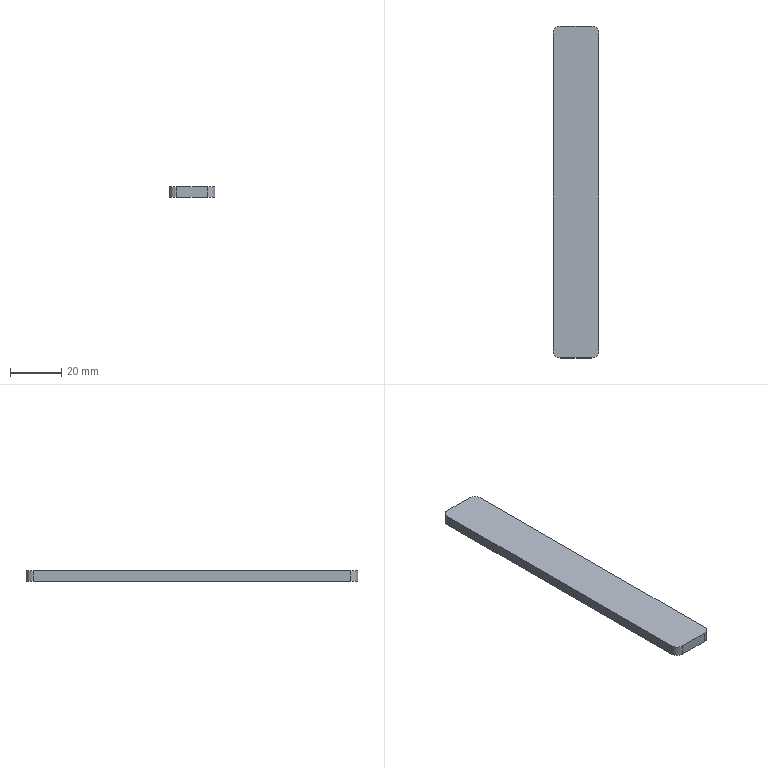Part | STEP file | 001-004-Feeding mechanism push plate | 1 solid | 10 faces | box 18 x 130 x 4 mm | volume 9329 mm3 | plane 6 | cylinder 4 | commonest cylinder face diameters 6 x4
STEP:
#1=CARTESIAN_POINT('',(0.,0.,0.));
#2=DIRECTION('',(0.,0.,1.));
#3=DIRECTION('',(1.,0.,0.));
#4=AXIS2_PLACEMENT_3D('',#1,#2,#3);
#5=CARTESIAN_POINT('',(9.,-62.,4.));
#6=VERTEX_POINT('',#5);
#7=CARTESIAN_POINT('',(9.,62.,4.));
#8=VERTEX_POINT('',#7);
#9=CARTESIAN_POINT('',(9.,-65.,4.));
#10=DIRECTION('',(0.,1.,0.));
#11=VECTOR('',#10,1.);
#12=LINE('',#9,#11);
#13=CARTESIAN_POINT('',(9.,-65.,4.));
#14=DIRECTION('',(-1.,0.,0.));
#15=DIRECTION('',(0.,0.,1.));
#16=AXIS2_PLACEMENT_3D('',#13,#14,#15);
#17=PLANE('',#16);
#18=CARTESIAN_POINT('',(0.,0.));
#19=DIRECTION('',(0.,1.));
#20=VECTOR('',#19,1.);
#21=LINE('',#18,#20);
#22=(GEOMETRIC_REPRESENTATION_CONTEXT(2)PARAMETRIC_REPRESENTATION_CONTEXT()REPRESENTATION_CONTEXT('',''));
#23=DEFINITIONAL_REPRESENTATION('',(#21),#22);
#24=PCURVE('',#17,#23);
#25=CARTESIAN_POINT('',(0.,0.,4.));
#26=DIRECTION('',(0.,0.,-1.));
#27=DIRECTION('',(-1.,0.,0.));
#28=AXIS2_PLACEMENT_3D('',#25,#26,#27);
#29=PLANE('',#28);
#30=CARTESIAN_POINT('',(-9.,-65.));
#31=DIRECTION('',(0.,1.));
#32=VECTOR('',#31,1.);
#33=LINE('',#30,#32);
#34=(GEOMETRIC_REPRESENTATION_CONTEXT(2)PARAMETRIC_REPRESENTATION_CONTEXT()REPRESENTATION_CONTEXT('',''));
#35=DEFINITIONAL_REPRESENTATION('',(#33),#34);
#36=PCURVE('',#29,#35);
#37=SURFACE_CURVE('',#12,(#24,#36),.PCURVE_S1.);
#38=EDGE_CURVE('',#6,#8,#37,.T.);
#39=ORIENTED_EDGE('',*,*,#38,.F.);
#40=CARTESIAN_POINT('',(9.,-62.,0.));
#41=VERTEX_POINT('',#40);
#42=CARTESIAN_POINT('',(9.,-62.,4.));
#43=DIRECTION('',(0.,0.,-1.));
#44=VECTOR('',#43,1.);
#45=LINE('',#42,#44);
#46=CARTESIAN_POINT('',(0.,3.));
#47=DIRECTION('',(-1.,0.));
#48=VECTOR('',#47,1.);
#49=LINE('',#46,#48);
#50=(GEOMETRIC_REPRESENTATION_CONTEXT(2)PARAMETRIC_REPRESENTATION_CONTEXT()REPRESENTATION_CONTEXT('',''));
#51=DEFINITIONAL_REPRESENTATION('',(#49),#50);
#52=PCURVE('',#17,#51);
#53=CARTESIAN_POINT('',(6.,-62.,4.));
#54=DIRECTION('',(0.,0.,-1.));
#55=DIRECTION('',(-1.,0.,0.));
#56=AXIS2_PLACEMENT_3D('',#53,#54,#55);
#57=CYLINDRICAL_SURFACE('',#56,3.);
#58=CARTESIAN_POINT('',(3.142,0.));
#59=DIRECTION('',(0.,1.));
#60=VECTOR('',#59,1.);
#61=LINE('',#58,#60);
#62=(GEOMETRIC_REPRESENTATION_CONTEXT(2)PARAMETRIC_REPRESENTATION_CONTEXT()REPRESENTATION_CONTEXT('',''));
#63=DEFINITIONAL_REPRESENTATION('',(#61),#62);
#64=PCURVE('',#57,#63);
#65=SURFACE_CURVE('',#45,(#52,#64),.PCURVE_S1.);
#66=EDGE_CURVE('',#6,#41,#65,.T.);
#67=ORIENTED_EDGE('',*,*,#66,.T.);
#68=CARTESIAN_POINT('',(9.,62.,0.));
#69=VERTEX_POINT('',#68);
#70=CARTESIAN_POINT('',(9.,-65.,0.));
#71=DIRECTION('',(0.,1.,0.));
#72=VECTOR('',#71,1.);
#73=LINE('',#70,#72);
#74=CARTESIAN_POINT('',(-4.,0.));
#75=DIRECTION('',(0.,1.));
#76=VECTOR('',#75,1.);
#77=LINE('',#74,#76);
#78=(GEOMETRIC_REPRESENTATION_CONTEXT(2)PARAMETRIC_REPRESENTATION_CONTEXT()REPRESENTATION_CONTEXT('',''));
#79=DEFINITIONAL_REPRESENTATION('',(#77),#78);
#80=PCURVE('',#17,#79);
#81=CARTESIAN_POINT('',(0.,0.,0.));
#82=DIRECTION('',(0.,0.,-1.));
#83=DIRECTION('',(-1.,0.,0.));
#84=AXIS2_PLACEMENT_3D('',#81,#82,#83);
#85=PLANE('',#84);
#86=CARTESIAN_POINT('',(-9.,-65.));
#87=DIRECTION('',(0.,1.));
#88=VECTOR('',#87,1.);
#89=LINE('',#86,#88);
#90=(GEOMETRIC_REPRESENTATION_CONTEXT(2)PARAMETRIC_REPRESENTATION_CONTEXT()REPRESENTATION_CONTEXT('',''));
#91=DEFINITIONAL_REPRESENTATION('',(#89),#90);
#92=PCURVE('',#85,#91);
#93=SURFACE_CURVE('',#73,(#80,#92),.PCURVE_S1.);
#94=EDGE_CURVE('',#41,#69,#93,.T.);
#95=ORIENTED_EDGE('',*,*,#94,.T.);
#96=CARTESIAN_POINT('',(9.,62.,4.));
#97=DIRECTION('',(0.,0.,1.));
#98=VECTOR('',#97,1.);
#99=LINE('',#96,#98);
#100=CARTESIAN_POINT('',(0.,127.));
#101=DIRECTION('',(1.,0.));
#102=VECTOR('',#101,1.);
#103=LINE('',#100,#102);
#104=(GEOMETRIC_REPRESENTATION_CONTEXT(2)PARAMETRIC_REPRESENTATION_CONTEXT()REPRESENTATION_CONTEXT('',''));
#105=DEFINITIONAL_REPRESENTATION('',(#103),#104);
#106=PCURVE('',#17,#105);
#107=CARTESIAN_POINT('',(6.,62.,4.));
#108=DIRECTION('',(0.,0.,-1.));
#109=DIRECTION('',(-1.,0.,0.));
#110=AXIS2_PLACEMENT_3D('',#107,#108,#109);
#111=CYLINDRICAL_SURFACE('',#110,3.);
#112=CARTESIAN_POINT('',(3.142,0.));
#113=DIRECTION('',(0.,-1.));
#114=VECTOR('',#113,1.);
#115=LINE('',#112,#114);
#116=(GEOMETRIC_REPRESENTATION_CONTEXT(2)PARAMETRIC_REPRESENTATION_CONTEXT()REPRESENTATION_CONTEXT('',''));
#117=DEFINITIONAL_REPRESENTATION('',(#115),#116);
#118=PCURVE('',#111,#117);
#119=SURFACE_CURVE('',#99,(#106,#118),.PCURVE_S1.);
#120=EDGE_CURVE('',#69,#8,#119,.T.);
#121=ORIENTED_EDGE('',*,*,#120,.T.);
#122=EDGE_LOOP('',(#39,#67,#95,#121));
#123=FACE_BOUND('',#122,.T.);
#124=ADVANCED_FACE('',(#123),#17,.F.);
#125=CARTESIAN_POINT('',(6.,65.,0.));
#126=VERTEX_POINT('',#125);
#127=CARTESIAN_POINT('',(-6.,65.,0.));
#128=VERTEX_POINT('',#127);
#129=CARTESIAN_POINT('',(-9.,65.,0.));
#130=DIRECTION('',(-1.,0.,0.));
#131=VECTOR('',#130,1.);
#132=LINE('',#129,#131);
#133=CARTESIAN_POINT('',(-9.,65.,4.));
#134=DIRECTION('',(0.,-1.,0.));
#135=DIRECTION('',(0.,0.,-1.));
#136=AXIS2_PLACEMENT_3D('',#133,#134,#135);
#137=PLANE('',#136);
#138=CARTESIAN_POINT('',(4.,0.));
#139=DIRECTION('',(0.,-1.));
#140=VECTOR('',#139,1.);
#141=LINE('',#138,#140);
#142=(GEOMETRIC_REPRESENTATION_CONTEXT(2)PARAMETRIC_REPRESENTATION_CONTEXT()REPRESENTATION_CONTEXT('',''));
#143=DEFINITIONAL_REPRESENTATION('',(#141),#142);
#144=PCURVE('',#137,#143);
#145=CARTESIAN_POINT('',(9.,65.));
#146=DIRECTION('',(1.,0.));
#147=VECTOR('',#146,1.);
#148=LINE('',#145,#147);
#149=(GEOMETRIC_REPRESENTATION_CONTEXT(2)PARAMETRIC_REPRESENTATION_CONTEXT()REPRESENTATION_CONTEXT('',''));
#150=DEFINITIONAL_REPRESENTATION('',(#148),#149);
#151=PCURVE('',#85,#150);
#152=SURFACE_CURVE('',#132,(#144,#151),.PCURVE_S1.);
#153=EDGE_CURVE('',#126,#128,#152,.T.);
#154=ORIENTED_EDGE('',*,*,#153,.T.);
#155=CARTESIAN_POINT('',(-6.,65.,4.));
#156=VERTEX_POINT('',#155);
#157=CARTESIAN_POINT('',(-6.,65.,4.));
#158=DIRECTION('',(0.,0.,1.));
#159=VECTOR('',#158,1.);
#160=LINE('',#157,#159);
#161=CARTESIAN_POINT('',(0.,3.));
#162=DIRECTION('',(-1.,0.));
#163=VECTOR('',#162,1.);
#164=LINE('',#161,#163);
#165=(GEOMETRIC_REPRESENTATION_CONTEXT(2)PARAMETRIC_REPRESENTATION_CONTEXT()REPRESENTATION_CONTEXT('',''));
#166=DEFINITIONAL_REPRESENTATION('',(#164),#165);
#167=PCURVE('',#137,#166);
#168=CARTESIAN_POINT('',(-6.,62.,4.));
#169=DIRECTION('',(0.,0.,-1.));
#170=DIRECTION('',(-1.,0.,0.));
#171=AXIS2_PLACEMENT_3D('',#168,#169,#170);
#172=CYLINDRICAL_SURFACE('',#171,3.);
#173=CARTESIAN_POINT('',(1.571,0.));
#174=DIRECTION('',(0.,-1.));
#175=VECTOR('',#174,1.);
#176=LINE('',#173,#175);
#177=(GEOMETRIC_REPRESENTATION_CONTEXT(2)PARAMETRIC_REPRESENTATION_CONTEXT()REPRESENTATION_CONTEXT('',''));
#178=DEFINITIONAL_REPRESENTATION('',(#176),#177);
#179=PCURVE('',#172,#178);
#180=SURFACE_CURVE('',#160,(#167,#179),.PCURVE_S1.);
#181=EDGE_CURVE('',#128,#156,#180,.T.);
#182=ORIENTED_EDGE('',*,*,#181,.T.);
#183=CARTESIAN_POINT('',(6.,65.,4.));
#184=VERTEX_POINT('',#183);
#185=CARTESIAN_POINT('',(-9.,65.,4.));
#186=DIRECTION('',(-1.,0.,0.));
#187=VECTOR('',#186,1.);
#188=LINE('',#185,#187);
#189=CARTESIAN_POINT('',(0.,0.));
#190=DIRECTION('',(0.,-1.));
#191=VECTOR('',#190,1.);
#192=LINE('',#189,#191);
#193=(GEOMETRIC_REPRESENTATION_CONTEXT(2)PARAMETRIC_REPRESENTATION_CONTEXT()REPRESENTATION_CONTEXT('',''));
#194=DEFINITIONAL_REPRESENTATION('',(#192),#193);
#195=PCURVE('',#137,#194);
#196=CARTESIAN_POINT('',(9.,65.));
#197=DIRECTION('',(1.,0.));
#198=VECTOR('',#197,1.);
#199=LINE('',#196,#198);
#200=(GEOMETRIC_REPRESENTATION_CONTEXT(2)PARAMETRIC_REPRESENTATION_CONTEXT()REPRESENTATION_CONTEXT('',''));
#201=DEFINITIONAL_REPRESENTATION('',(#199),#200);
#202=PCURVE('',#29,#201);
#203=SURFACE_CURVE('',#188,(#195,#202),.PCURVE_S1.);
#204=EDGE_CURVE('',#184,#156,#203,.T.);
#205=ORIENTED_EDGE('',*,*,#204,.F.);
#206=CARTESIAN_POINT('',(6.,65.,4.));
#207=DIRECTION('',(0.,0.,-1.));
#208=VECTOR('',#207,1.);
#209=LINE('',#206,#208);
#210=CARTESIAN_POINT('',(0.,15.));
#211=DIRECTION('',(1.,0.));
#212=VECTOR('',#211,1.);
#213=LINE('',#210,#212);
#214=(GEOMETRIC_REPRESENTATION_CONTEXT(2)PARAMETRIC_REPRESENTATION_CONTEXT()REPRESENTATION_CONTEXT('',''));
#215=DEFINITIONAL_REPRESENTATION('',(#213),#214);
#216=PCURVE('',#137,#215);
#217=CARTESIAN_POINT('',(1.571,0.));
#218=DIRECTION('',(0.,1.));
#219=VECTOR('',#218,1.);
#220=LINE('',#217,#219);
#221=(GEOMETRIC_REPRESENTATION_CONTEXT(2)PARAMETRIC_REPRESENTATION_CONTEXT()REPRESENTATION_CONTEXT('',''));
#222=DEFINITIONAL_REPRESENTATION('',(#220),#221);
#223=PCURVE('',#111,#222);
#224=SURFACE_CURVE('',#209,(#216,#223),.PCURVE_S1.);
#225=EDGE_CURVE('',#184,#126,#224,.T.);
#226=ORIENTED_EDGE('',*,*,#225,.T.);
#227=EDGE_LOOP('',(#154,#182,#205,#226));
#228=FACE_BOUND('',#227,.T.);
#229=ADVANCED_FACE('',(#228),#137,.F.);
#230=CARTESIAN_POINT('',(-9.,62.,0.));
#231=VERTEX_POINT('',#230);
#232=CARTESIAN_POINT('',(-9.,-62.,0.));
#233=VERTEX_POINT('',#232);
#234=CARTESIAN_POINT('',(-9.,-65.,0.));
#235=DIRECTION('',(0.,-1.,0.));
#236=VECTOR('',#235,1.);
#237=LINE('',#234,#236);
#238=CARTESIAN_POINT('',(-9.,-65.,4.));
#239=DIRECTION('',(1.,0.,0.));
#240=DIRECTION('',(0.,0.,-1.));
#241=AXIS2_PLACEMENT_3D('',#238,#239,#240);
#242=PLANE('',#241);
#243=CARTESIAN_POINT('',(4.,0.));
#244=DIRECTION('',(0.,-1.));
#245=VECTOR('',#244,1.);
#246=LINE('',#243,#245);
#247=(GEOMETRIC_REPRESENTATION_CONTEXT(2)PARAMETRIC_REPRESENTATION_CONTEXT()REPRESENTATION_CONTEXT('',''));
#248=DEFINITIONAL_REPRESENTATION('',(#246),#247);
#249=PCURVE('',#242,#248);
#250=CARTESIAN_POINT('',(9.,-65.));
#251=DIRECTION('',(0.,-1.));
#252=VECTOR('',#251,1.);
#253=LINE('',#250,#252);
#254=(GEOMETRIC_REPRESENTATION_CONTEXT(2)PARAMETRIC_REPRESENTATION_CONTEXT()REPRESENTATION_CONTEXT('',''));
#255=DEFINITIONAL_REPRESENTATION('',(#253),#254);
#256=PCURVE('',#85,#255);
#257=SURFACE_CURVE('',#237,(#249,#256),.PCURVE_S1.);
#258=EDGE_CURVE('',#231,#233,#257,.T.);
#259=ORIENTED_EDGE('',*,*,#258,.T.);
#260=CARTESIAN_POINT('',(-9.,-62.,4.));
#261=VERTEX_POINT('',#260);
#262=CARTESIAN_POINT('',(-9.,-62.,4.));
#263=DIRECTION('',(0.,0.,1.));
#264=VECTOR('',#263,1.);
#265=LINE('',#262,#264);
#266=CARTESIAN_POINT('',(0.,3.));
#267=DIRECTION('',(-1.,0.));
#268=VECTOR('',#267,1.);
#269=LINE('',#266,#268);
#270=(GEOMETRIC_REPRESENTATION_CONTEXT(2)PARAMETRIC_REPRESENTATION_CONTEXT()REPRESENTATION_CONTEXT('',''));
#271=DEFINITIONAL_REPRESENTATION('',(#269),#270);
#272=PCURVE('',#242,#271);
#273=CARTESIAN_POINT('',(-6.,-62.,4.));
#274=DIRECTION('',(0.,0.,-1.));
#275=DIRECTION('',(-1.,0.,0.));
#276=AXIS2_PLACEMENT_3D('',#273,#274,#275);
#277=CYLINDRICAL_SURFACE('',#276,3.);
#278=CARTESIAN_POINT('',(6.283,0.));
#279=DIRECTION('',(0.,-1.));
#280=VECTOR('',#279,1.);
#281=LINE('',#278,#280);
#282=(GEOMETRIC_REPRESENTATION_CONTEXT(2)PARAMETRIC_REPRESENTATION_CONTEXT()REPRESENTATION_CONTEXT('',''));
#283=DEFINITIONAL_REPRESENTATION('',(#281),#282);
#284=PCURVE('',#277,#283);
#285=SURFACE_CURVE('',#265,(#272,#284),.PCURVE_S1.);
#286=EDGE_CURVE('',#233,#261,#285,.T.);
#287=ORIENTED_EDGE('',*,*,#286,.T.);
#288=CARTESIAN_POINT('',(-9.,62.,4.));
#289=VERTEX_POINT('',#288);
#290=CARTESIAN_POINT('',(-9.,-65.,4.));
#291=DIRECTION('',(0.,-1.,0.));
#292=VECTOR('',#291,1.);
#293=LINE('',#290,#292);
#294=CARTESIAN_POINT('',(0.,0.));
#295=DIRECTION('',(0.,-1.));
#296=VECTOR('',#295,1.);
#297=LINE('',#294,#296);
#298=(GEOMETRIC_REPRESENTATION_CONTEXT(2)PARAMETRIC_REPRESENTATION_CONTEXT()REPRESENTATION_CONTEXT('',''));
#299=DEFINITIONAL_REPRESENTATION('',(#297),#298);
#300=PCURVE('',#242,#299);
#301=CARTESIAN_POINT('',(9.,-65.));
#302=DIRECTION('',(0.,-1.));
#303=VECTOR('',#302,1.);
#304=LINE('',#301,#303);
#305=(GEOMETRIC_REPRESENTATION_CONTEXT(2)PARAMETRIC_REPRESENTATION_CONTEXT()REPRESENTATION_CONTEXT('',''));
#306=DEFINITIONAL_REPRESENTATION('',(#304),#305);
#307=PCURVE('',#29,#306);
#308=SURFACE_CURVE('',#293,(#300,#307),.PCURVE_S1.);
#309=EDGE_CURVE('',#289,#261,#308,.T.);
#310=ORIENTED_EDGE('',*,*,#309,.F.);
#311=CARTESIAN_POINT('',(-9.,62.,4.));
#312=DIRECTION('',(0.,0.,-1.));
#313=VECTOR('',#312,1.);
#314=LINE('',#311,#313);
#315=CARTESIAN_POINT('',(0.,127.));
#316=DIRECTION('',(1.,0.));
#317=VECTOR('',#316,1.);
#318=LINE('',#315,#317);
#319=(GEOMETRIC_REPRESENTATION_CONTEXT(2)PARAMETRIC_REPRESENTATION_CONTEXT()REPRESENTATION_CONTEXT('',''));
#320=DEFINITIONAL_REPRESENTATION('',(#318),#319);
#321=PCURVE('',#242,#320);
#322=CARTESIAN_POINT('',(0.,0.));
#323=DIRECTION('',(0.,1.));
#324=VECTOR('',#323,1.);
#325=LINE('',#322,#324);
#326=(GEOMETRIC_REPRESENTATION_CONTEXT(2)PARAMETRIC_REPRESENTATION_CONTEXT()REPRESENTATION_CONTEXT('',''));
#327=DEFINITIONAL_REPRESENTATION('',(#325),#326);
#328=PCURVE('',#172,#327);
#329=SURFACE_CURVE('',#314,(#321,#328),.PCURVE_S1.);
#330=EDGE_CURVE('',#289,#231,#329,.T.);
#331=ORIENTED_EDGE('',*,*,#330,.T.);
#332=EDGE_LOOP('',(#259,#287,#310,#331));
#333=FACE_BOUND('',#332,.T.);
#334=ADVANCED_FACE('',(#333),#242,.F.);
#335=CARTESIAN_POINT('',(-6.,-65.,0.));
#336=VERTEX_POINT('',#335);
#337=CARTESIAN_POINT('',(6.,-65.,0.));
#338=VERTEX_POINT('',#337);
#339=CARTESIAN_POINT('',(-9.,-65.,0.));
#340=DIRECTION('',(1.,0.,0.));
#341=VECTOR('',#340,1.);
#342=LINE('',#339,#341);
#343=CARTESIAN_POINT('',(-9.,-65.,4.));
#344=DIRECTION('',(0.,1.,0.));
#345=DIRECTION('',(0.,0.,1.));
#346=AXIS2_PLACEMENT_3D('',#343,#344,#345);
#347=PLANE('',#346);
#348=CARTESIAN_POINT('',(-4.,0.));
#349=DIRECTION('',(0.,1.));
#350=VECTOR('',#349,1.);
#351=LINE('',#348,#350);
#352=(GEOMETRIC_REPRESENTATION_CONTEXT(2)PARAMETRIC_REPRESENTATION_CONTEXT()REPRESENTATION_CONTEXT('',''));
#353=DEFINITIONAL_REPRESENTATION('',(#351),#352);
#354=PCURVE('',#347,#353);
#355=CARTESIAN_POINT('',(9.,-65.));
#356=DIRECTION('',(-1.,0.));
#357=VECTOR('',#356,1.);
#358=LINE('',#355,#357);
#359=(GEOMETRIC_REPRESENTATION_CONTEXT(2)PARAMETRIC_REPRESENTATION_CONTEXT()REPRESENTATION_CONTEXT('',''));
#360=DEFINITIONAL_REPRESENTATION('',(#358),#359);
#361=PCURVE('',#85,#360);
#362=SURFACE_CURVE('',#342,(#354,#361),.PCURVE_S1.);
#363=EDGE_CURVE('',#336,#338,#362,.T.);
#364=ORIENTED_EDGE('',*,*,#363,.T.);
#365=CARTESIAN_POINT('',(6.,-65.,4.));
#366=VERTEX_POINT('',#365);
#367=CARTESIAN_POINT('',(6.,-65.,4.));
#368=DIRECTION('',(0.,0.,1.));
#369=VECTOR('',#368,1.);
#370=LINE('',#367,#369);
#371=CARTESIAN_POINT('',(0.,15.));
#372=DIRECTION('',(1.,0.));
#373=VECTOR('',#372,1.);
#374=LINE('',#371,#373);
#375=(GEOMETRIC_REPRESENTATION_CONTEXT(2)PARAMETRIC_REPRESENTATION_CONTEXT()REPRESENTATION_CONTEXT('',''));
#376=DEFINITIONAL_REPRESENTATION('',(#374),#375);
#377=PCURVE('',#347,#376);
#378=CARTESIAN_POINT('',(4.712,0.));
#379=DIRECTION('',(0.,-1.));
#380=VECTOR('',#379,1.);
#381=LINE('',#378,#380);
#382=(GEOMETRIC_REPRESENTATION_CONTEXT(2)PARAMETRIC_REPRESENTATION_CONTEXT()REPRESENTATION_CONTEXT('',''));
#383=DEFINITIONAL_REPRESENTATION('',(#381),#382);
#384=PCURVE('',#57,#383);
#385=SURFACE_CURVE('',#370,(#377,#384),.PCURVE_S1.);
#386=EDGE_CURVE('',#338,#366,#385,.T.);
#387=ORIENTED_EDGE('',*,*,#386,.T.);
#388=CARTESIAN_POINT('',(-6.,-65.,4.));
#389=VERTEX_POINT('',#388);
#390=CARTESIAN_POINT('',(-9.,-65.,4.));
#391=DIRECTION('',(1.,0.,0.));
#392=VECTOR('',#391,1.);
#393=LINE('',#390,#392);
#394=CARTESIAN_POINT('',(0.,0.));
#395=DIRECTION('',(0.,1.));
#396=VECTOR('',#395,1.);
#397=LINE('',#394,#396);
#398=(GEOMETRIC_REPRESENTATION_CONTEXT(2)PARAMETRIC_REPRESENTATION_CONTEXT()REPRESENTATION_CONTEXT('',''));
#399=DEFINITIONAL_REPRESENTATION('',(#397),#398);
#400=PCURVE('',#347,#399);
#401=CARTESIAN_POINT('',(9.,-65.));
#402=DIRECTION('',(-1.,0.));
#403=VECTOR('',#402,1.);
#404=LINE('',#401,#403);
#405=(GEOMETRIC_REPRESENTATION_CONTEXT(2)PARAMETRIC_REPRESENTATION_CONTEXT()REPRESENTATION_CONTEXT('',''));
#406=DEFINITIONAL_REPRESENTATION('',(#404),#405);
#407=PCURVE('',#29,#406);
#408=SURFACE_CURVE('',#393,(#400,#407),.PCURVE_S1.);
#409=EDGE_CURVE('',#389,#366,#408,.T.);
#410=ORIENTED_EDGE('',*,*,#409,.F.);
#411=CARTESIAN_POINT('',(-6.,-65.,4.));
#412=DIRECTION('',(0.,0.,-1.));
#413=VECTOR('',#412,1.);
#414=LINE('',#411,#413);
#415=CARTESIAN_POINT('',(0.,3.));
#416=DIRECTION('',(-1.,0.));
#417=VECTOR('',#416,1.);
#418=LINE('',#415,#417);
#419=(GEOMETRIC_REPRESENTATION_CONTEXT(2)PARAMETRIC_REPRESENTATION_CONTEXT()REPRESENTATION_CONTEXT('',''));
#420=DEFINITIONAL_REPRESENTATION('',(#418),#419);
#421=PCURVE('',#347,#420);
#422=CARTESIAN_POINT('',(4.712,0.));
#423=DIRECTION('',(0.,1.));
#424=VECTOR('',#423,1.);
#425=LINE('',#422,#424);
#426=(GEOMETRIC_REPRESENTATION_CONTEXT(2)PARAMETRIC_REPRESENTATION_CONTEXT()REPRESENTATION_CONTEXT('',''));
#427=DEFINITIONAL_REPRESENTATION('',(#425),#426);
#428=PCURVE('',#277,#427);
#429=SURFACE_CURVE('',#414,(#421,#428),.PCURVE_S1.);
#430=EDGE_CURVE('',#389,#336,#429,.T.);
#431=ORIENTED_EDGE('',*,*,#430,.T.);
#432=EDGE_LOOP('',(#364,#387,#410,#431));
#433=FACE_BOUND('',#432,.T.);
#434=ADVANCED_FACE('',(#433),#347,.F.);
#435=ORIENTED_EDGE('',*,*,#409,.T.);
#436=CARTESIAN_POINT('',(6.,-62.,4.));
#437=DIRECTION('',(0.,0.,1.));
#438=DIRECTION('',(-1.,0.,0.));
#439=AXIS2_PLACEMENT_3D('',#436,#437,#438);
#440=CIRCLE('',#439,3.);
#441=CARTESIAN_POINT('',(-3.,-62.));
#442=CARTESIAN_POINT('',(-3.,-67.196));
#443=CARTESIAN_POINT('',(-7.5,-64.598));
#444=CARTESIAN_POINT('',(-12.,-62.));
#445=CARTESIAN_POINT('',(-7.5,-59.402));
#446=CARTESIAN_POINT('',(-3.,-56.804));
#447=CARTESIAN_POINT('',(-3.,-62.));
#448=(BOUNDED_CURVE()B_SPLINE_CURVE(2,(#441,#442,#443,#444,#445,#446,#447),.UNSPECIFIED.,.T.,.F.)B_SPLINE_CURVE_WITH_KNOTS((1,2,2,2,2,1),(-2.094,0.,2.094,4.189,6.283,8.378),.UNSPECIFIED.)CURVE()GEOMETRIC_REPRESENTATION_ITEM()RATIONAL_B_SPLINE_CURVE((1.,0.5,1.,0.5,1.,0.5,1.))REPRESENTATION_ITEM(''));
#449=(GEOMETRIC_REPRESENTATION_CONTEXT(2)PARAMETRIC_REPRESENTATION_CONTEXT()REPRESENTATION_CONTEXT('',''));
#450=DEFINITIONAL_REPRESENTATION('',(#448),#449);
#451=PCURVE('',#29,#450);
#452=CARTESIAN_POINT('',(6.283,0.));
#453=DIRECTION('',(-1.,0.));
#454=VECTOR('',#453,1.);
#455=LINE('',#452,#454);
#456=(GEOMETRIC_REPRESENTATION_CONTEXT(2)PARAMETRIC_REPRESENTATION_CONTEXT()REPRESENTATION_CONTEXT('',''));
#457=DEFINITIONAL_REPRESENTATION('',(#455),#456);
#458=PCURVE('',#57,#457);
#459=SURFACE_CURVE('',#440,(#451,#458),.PCURVE_S1.);
#460=EDGE_CURVE('',#366,#6,#459,.T.);
#461=ORIENTED_EDGE('',*,*,#460,.T.);
#462=ORIENTED_EDGE('',*,*,#38,.T.);
#463=CARTESIAN_POINT('',(6.,62.,4.));
#464=DIRECTION('',(0.,0.,1.));
#465=DIRECTION('',(-1.,0.,0.));
#466=AXIS2_PLACEMENT_3D('',#463,#464,#465);
#467=CIRCLE('',#466,3.);
#468=CARTESIAN_POINT('',(-3.,62.));
#469=CARTESIAN_POINT('',(-3.,56.804));
#470=CARTESIAN_POINT('',(-7.5,59.402));
#471=CARTESIAN_POINT('',(-12.,62.));
#472=CARTESIAN_POINT('',(-7.5,64.598));
#473=CARTESIAN_POINT('',(-3.,67.196));
#474=CARTESIAN_POINT('',(-3.,62.));
#475=(BOUNDED_CURVE()B_SPLINE_CURVE(2,(#468,#469,#470,#471,#472,#473,#474),.UNSPECIFIED.,.T.,.F.)B_SPLINE_CURVE_WITH_KNOTS((1,2,2,2,2,1),(-2.094,0.,2.094,4.189,6.283,8.378),.UNSPECIFIED.)CURVE()GEOMETRIC_REPRESENTATION_ITEM()RATIONAL_B_SPLINE_CURVE((1.,0.5,1.,0.5,1.,0.5,1.))REPRESENTATION_ITEM(''));
#476=(GEOMETRIC_REPRESENTATION_CONTEXT(2)PARAMETRIC_REPRESENTATION_CONTEXT()REPRESENTATION_CONTEXT('',''));
#477=DEFINITIONAL_REPRESENTATION('',(#475),#476);
#478=PCURVE('',#29,#477);
#479=CARTESIAN_POINT('',(6.283,0.));
#480=DIRECTION('',(-1.,0.));
#481=VECTOR('',#480,1.);
#482=LINE('',#479,#481);
#483=(GEOMETRIC_REPRESENTATION_CONTEXT(2)PARAMETRIC_REPRESENTATION_CONTEXT()REPRESENTATION_CONTEXT('',''));
#484=DEFINITIONAL_REPRESENTATION('',(#482),#483);
#485=PCURVE('',#111,#484);
#486=SURFACE_CURVE('',#467,(#478,#485),.PCURVE_S1.);
#487=EDGE_CURVE('',#8,#184,#486,.T.);
#488=ORIENTED_EDGE('',*,*,#487,.T.);
#489=ORIENTED_EDGE('',*,*,#204,.T.);
#490=CARTESIAN_POINT('',(-6.,62.,4.));
#491=DIRECTION('',(0.,0.,1.));
#492=DIRECTION('',(-1.,0.,0.));
#493=AXIS2_PLACEMENT_3D('',#490,#491,#492);
#494=CIRCLE('',#493,3.);
#495=CARTESIAN_POINT('',(9.,62.));
#496=CARTESIAN_POINT('',(9.,56.804));
#497=CARTESIAN_POINT('',(4.5,59.402));
#498=CARTESIAN_POINT('',(0.,62.));
#499=CARTESIAN_POINT('',(4.5,64.598));
#500=CARTESIAN_POINT('',(9.,67.196));
#501=CARTESIAN_POINT('',(9.,62.));
#502=(BOUNDED_CURVE()B_SPLINE_CURVE(2,(#495,#496,#497,#498,#499,#500,#501),.UNSPECIFIED.,.T.,.F.)B_SPLINE_CURVE_WITH_KNOTS((1,2,2,2,2,1),(-2.094,0.,2.094,4.189,6.283,8.378),.UNSPECIFIED.)CURVE()GEOMETRIC_REPRESENTATION_ITEM()RATIONAL_B_SPLINE_CURVE((1.,0.5,1.,0.5,1.,0.5,1.))REPRESENTATION_ITEM(''));
#503=(GEOMETRIC_REPRESENTATION_CONTEXT(2)PARAMETRIC_REPRESENTATION_CONTEXT()REPRESENTATION_CONTEXT('',''));
#504=DEFINITIONAL_REPRESENTATION('',(#502),#503);
#505=PCURVE('',#29,#504);
#506=CARTESIAN_POINT('',(6.283,0.));
#507=DIRECTION('',(-1.,0.));
#508=VECTOR('',#507,1.);
#509=LINE('',#506,#508);
#510=(GEOMETRIC_REPRESENTATION_CONTEXT(2)PARAMETRIC_REPRESENTATION_CONTEXT()REPRESENTATION_CONTEXT('',''));
#511=DEFINITIONAL_REPRESENTATION('',(#509),#510);
#512=PCURVE('',#172,#511);
#513=SURFACE_CURVE('',#494,(#505,#512),.PCURVE_S1.);
#514=EDGE_CURVE('',#156,#289,#513,.T.);
#515=ORIENTED_EDGE('',*,*,#514,.T.);
#516=ORIENTED_EDGE('',*,*,#309,.T.);
#517=CARTESIAN_POINT('',(-6.,-62.,4.));
#518=DIRECTION('',(0.,0.,1.));
#519=DIRECTION('',(-1.,0.,0.));
#520=AXIS2_PLACEMENT_3D('',#517,#518,#519);
#521=CIRCLE('',#520,3.);
#522=CARTESIAN_POINT('',(9.,-62.));
#523=CARTESIAN_POINT('',(9.,-67.196));
#524=CARTESIAN_POINT('',(4.5,-64.598));
#525=CARTESIAN_POINT('',(0.,-62.));
#526=CARTESIAN_POINT('',(4.5,-59.402));
#527=CARTESIAN_POINT('',(9.,-56.804));
#528=CARTESIAN_POINT('',(9.,-62.));
#529=(BOUNDED_CURVE()B_SPLINE_CURVE(2,(#522,#523,#524,#525,#526,#527,#528),.UNSPECIFIED.,.T.,.F.)B_SPLINE_CURVE_WITH_KNOTS((1,2,2,2,2,1),(-2.094,0.,2.094,4.189,6.283,8.378),.UNSPECIFIED.)CURVE()GEOMETRIC_REPRESENTATION_ITEM()RATIONAL_B_SPLINE_CURVE((1.,0.5,1.,0.5,1.,0.5,1.))REPRESENTATION_ITEM(''));
#530=(GEOMETRIC_REPRESENTATION_CONTEXT(2)PARAMETRIC_REPRESENTATION_CONTEXT()REPRESENTATION_CONTEXT('',''));
#531=DEFINITIONAL_REPRESENTATION('',(#529),#530);
#532=PCURVE('',#29,#531);
#533=CARTESIAN_POINT('',(6.283,0.));
#534=DIRECTION('',(-1.,0.));
#535=VECTOR('',#534,1.);
#536=LINE('',#533,#535);
#537=(GEOMETRIC_REPRESENTATION_CONTEXT(2)PARAMETRIC_REPRESENTATION_CONTEXT()REPRESENTATION_CONTEXT('',''));
#538=DEFINITIONAL_REPRESENTATION('',(#536),#537);
#539=PCURVE('',#277,#538);
#540=SURFACE_CURVE('',#521,(#532,#539),.PCURVE_S1.);
#541=EDGE_CURVE('',#261,#389,#540,.T.);
#542=ORIENTED_EDGE('',*,*,#541,.T.);
#543=EDGE_LOOP('',(#435,#461,#462,#488,#489,#515,#516,#542));
#544=FACE_BOUND('',#543,.T.);
#545=ADVANCED_FACE('',(#544),#29,.F.);
#546=ORIENTED_EDGE('',*,*,#94,.F.);
#547=CARTESIAN_POINT('',(6.,-62.,0.));
#548=DIRECTION('',(0.,0.,-1.));
#549=DIRECTION('',(-1.,0.,0.));
#550=AXIS2_PLACEMENT_3D('',#547,#548,#549);
#551=CIRCLE('',#550,3.);
#552=CARTESIAN_POINT('',(-6.,-62.));
#553=DIRECTION('',(1.,0.));
#554=AXIS2_PLACEMENT_2D('',#552,#553);
#555=CIRCLE('',#554,3.);
#556=(GEOMETRIC_REPRESENTATION_CONTEXT(2)PARAMETRIC_REPRESENTATION_CONTEXT()REPRESENTATION_CONTEXT('',''));
#557=DEFINITIONAL_REPRESENTATION('',(#555),#556);
#558=PCURVE('',#85,#557);
#559=CARTESIAN_POINT('',(0.,4.));
#560=DIRECTION('',(1.,0.));
#561=VECTOR('',#560,1.);
#562=LINE('',#559,#561);
#563=(GEOMETRIC_REPRESENTATION_CONTEXT(2)PARAMETRIC_REPRESENTATION_CONTEXT()REPRESENTATION_CONTEXT('',''));
#564=DEFINITIONAL_REPRESENTATION('',(#562),#563);
#565=PCURVE('',#57,#564);
#566=SURFACE_CURVE('',#551,(#558,#565),.PCURVE_S1.);
#567=EDGE_CURVE('',#41,#338,#566,.T.);
#568=ORIENTED_EDGE('',*,*,#567,.T.);
#569=ORIENTED_EDGE('',*,*,#363,.F.);
#570=CARTESIAN_POINT('',(-6.,-62.,0.));
#571=DIRECTION('',(0.,0.,-1.));
#572=DIRECTION('',(-1.,0.,0.));
#573=AXIS2_PLACEMENT_3D('',#570,#571,#572);
#574=CIRCLE('',#573,3.);
#575=CARTESIAN_POINT('',(6.,-62.));
#576=DIRECTION('',(1.,0.));
#577=AXIS2_PLACEMENT_2D('',#575,#576);
#578=CIRCLE('',#577,3.);
#579=(GEOMETRIC_REPRESENTATION_CONTEXT(2)PARAMETRIC_REPRESENTATION_CONTEXT()REPRESENTATION_CONTEXT('',''));
#580=DEFINITIONAL_REPRESENTATION('',(#578),#579);
#581=PCURVE('',#85,#580);
#582=CARTESIAN_POINT('',(0.,4.));
#583=DIRECTION('',(1.,0.));
#584=VECTOR('',#583,1.);
#585=LINE('',#582,#584);
#586=(GEOMETRIC_REPRESENTATION_CONTEXT(2)PARAMETRIC_REPRESENTATION_CONTEXT()REPRESENTATION_CONTEXT('',''));
#587=DEFINITIONAL_REPRESENTATION('',(#585),#586);
#588=PCURVE('',#277,#587);
#589=SURFACE_CURVE('',#574,(#581,#588),.PCURVE_S1.);
#590=EDGE_CURVE('',#336,#233,#589,.T.);
#591=ORIENTED_EDGE('',*,*,#590,.T.);
#592=ORIENTED_EDGE('',*,*,#258,.F.);
#593=CARTESIAN_POINT('',(-6.,62.,0.));
#594=DIRECTION('',(0.,0.,-1.));
#595=DIRECTION('',(-1.,0.,0.));
#596=AXIS2_PLACEMENT_3D('',#593,#594,#595);
#597=CIRCLE('',#596,3.);
#598=CARTESIAN_POINT('',(6.,62.));
#599=DIRECTION('',(1.,0.));
#600=AXIS2_PLACEMENT_2D('',#598,#599);
#601=CIRCLE('',#600,3.);
#602=(GEOMETRIC_REPRESENTATION_CONTEXT(2)PARAMETRIC_REPRESENTATION_CONTEXT()REPRESENTATION_CONTEXT('',''));
#603=DEFINITIONAL_REPRESENTATION('',(#601),#602);
#604=PCURVE('',#85,#603);
#605=CARTESIAN_POINT('',(0.,4.));
#606=DIRECTION('',(1.,0.));
#607=VECTOR('',#606,1.);
#608=LINE('',#605,#607);
#609=(GEOMETRIC_REPRESENTATION_CONTEXT(2)PARAMETRIC_REPRESENTATION_CONTEXT()REPRESENTATION_CONTEXT('',''));
#610=DEFINITIONAL_REPRESENTATION('',(#608),#609);
#611=PCURVE('',#172,#610);
#612=SURFACE_CURVE('',#597,(#604,#611),.PCURVE_S1.);
#613=EDGE_CURVE('',#231,#128,#612,.T.);
#614=ORIENTED_EDGE('',*,*,#613,.T.);
#615=ORIENTED_EDGE('',*,*,#153,.F.);
#616=CARTESIAN_POINT('',(6.,62.,0.));
#617=DIRECTION('',(0.,0.,-1.));
#618=DIRECTION('',(-1.,0.,0.));
#619=AXIS2_PLACEMENT_3D('',#616,#617,#618);
#620=CIRCLE('',#619,3.);
#621=CARTESIAN_POINT('',(-6.,62.));
#622=DIRECTION('',(1.,0.));
#623=AXIS2_PLACEMENT_2D('',#621,#622);
#624=CIRCLE('',#623,3.);
#625=(GEOMETRIC_REPRESENTATION_CONTEXT(2)PARAMETRIC_REPRESENTATION_CONTEXT()REPRESENTATION_CONTEXT('',''));
#626=DEFINITIONAL_REPRESENTATION('',(#624),#625);
#627=PCURVE('',#85,#626);
#628=CARTESIAN_POINT('',(0.,4.));
#629=DIRECTION('',(1.,0.));
#630=VECTOR('',#629,1.);
#631=LINE('',#628,#630);
#632=(GEOMETRIC_REPRESENTATION_CONTEXT(2)PARAMETRIC_REPRESENTATION_CONTEXT()REPRESENTATION_CONTEXT('',''));
#633=DEFINITIONAL_REPRESENTATION('',(#631),#632);
#634=PCURVE('',#111,#633);
#635=SURFACE_CURVE('',#620,(#627,#634),.PCURVE_S1.);
#636=EDGE_CURVE('',#126,#69,#635,.T.);
#637=ORIENTED_EDGE('',*,*,#636,.T.);
#638=EDGE_LOOP('',(#546,#568,#569,#591,#592,#614,#615,#637));
#639=FACE_BOUND('',#638,.T.);
#640=ADVANCED_FACE('',(#639),#85,.T.);
#641=ORIENTED_EDGE('',*,*,#460,.F.);
#642=ORIENTED_EDGE('',*,*,#386,.F.);
#643=ORIENTED_EDGE('',*,*,#567,.F.);
#644=ORIENTED_EDGE('',*,*,#66,.F.);
#645=EDGE_LOOP('',(#641,#642,#643,#644));
#646=FACE_BOUND('',#645,.T.);
#647=ADVANCED_FACE('',(#646),#57,.T.);
#648=ORIENTED_EDGE('',*,*,#541,.F.);
#649=ORIENTED_EDGE('',*,*,#286,.F.);
#650=ORIENTED_EDGE('',*,*,#590,.F.);
#651=ORIENTED_EDGE('',*,*,#430,.F.);
#652=EDGE_LOOP('',(#648,#649,#650,#651));
#653=FACE_BOUND('',#652,.T.);
#654=ADVANCED_FACE('',(#653),#277,.T.);
#655=ORIENTED_EDGE('',*,*,#514,.F.);
#656=ORIENTED_EDGE('',*,*,#181,.F.);
#657=ORIENTED_EDGE('',*,*,#613,.F.);
#658=ORIENTED_EDGE('',*,*,#330,.F.);
#659=EDGE_LOOP('',(#655,#656,#657,#658));
#660=FACE_BOUND('',#659,.T.);
#661=ADVANCED_FACE('',(#660),#172,.T.);
#662=ORIENTED_EDGE('',*,*,#487,.F.);
#663=ORIENTED_EDGE('',*,*,#120,.F.);
#664=ORIENTED_EDGE('',*,*,#636,.F.);
#665=ORIENTED_EDGE('',*,*,#225,.F.);
#666=EDGE_LOOP('',(#662,#663,#664,#665));
#667=FACE_BOUND('',#666,.T.);
#668=ADVANCED_FACE('',(#667),#111,.T.);
#669=CLOSED_SHELL('',(#124,#229,#334,#434,#545,#640,#647,#654,#661,#668));
#670=MANIFOLD_SOLID_BREP('',#669);
#671=(LENGTH_UNIT()NAMED_UNIT(*)SI_UNIT(.MILLI.,.METRE.));
#672=UNCERTAINTY_MEASURE_WITH_UNIT(LENGTH_MEASURE(0.0000001),#671,'','');
#673=(NAMED_UNIT(*)PLANE_ANGLE_UNIT()SI_UNIT($,.RADIAN.));
#674=(NAMED_UNIT(*)SI_UNIT($,.STERADIAN.)SOLID_ANGLE_UNIT());
#675=(GEOMETRIC_REPRESENTATION_CONTEXT(3)GLOBAL_UNCERTAINTY_ASSIGNED_CONTEXT((#672))GLOBAL_UNIT_ASSIGNED_CONTEXT((#671,#673,#674))REPRESENTATION_CONTEXT('',''));
#676=ADVANCED_BREP_SHAPE_REPRESENTATION('',(#4,#670),#675);